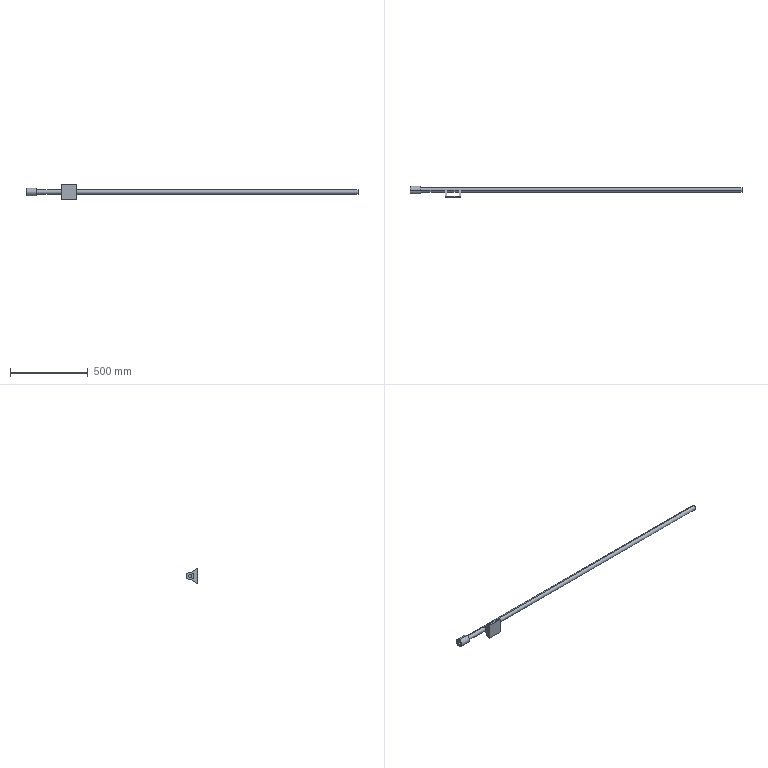Part | STEP file | Rail shaft | 1 solid | 24 faces | box 2134 x 75 x 100 mm | volume 1735049 mm3 | plane 16 | cylinder 8 | commonest cylinder face diameters 30 x4 20 x2 50 x2
STEP:
#1=CARTESIAN_POINT('',(-276.,50.,-10.));
#2=VERTEX_POINT('',#1);
#3=CARTESIAN_POINT('',(-276.,50.,10.));
#4=VERTEX_POINT('',#3);
#5=CARTESIAN_POINT('',(-276.,50.,0.));
#6=DIRECTION('',(-1.,0.,0.));
#7=DIRECTION('',(0.,0.,1.));
#8=AXIS2_PLACEMENT_3D('',#5,#6,#7);
#9=CIRCLE('',#8,10.);
#10=EDGE_CURVE('',#2,#4,#9,.T.);
#11=ORIENTED_EDGE('',*,*,#10,.T.);
#12=CARTESIAN_POINT('',(-256.,50.,10.));
#13=VERTEX_POINT('',#12);
#14=CARTESIAN_POINT('',(-276.,50.,10.));
#15=DIRECTION('',(1.,0.,0.));
#16=VECTOR('',#15,1000.);
#17=LINE('',#14,#16);
#18=EDGE_CURVE('',#4,#13,#17,.T.);
#19=ORIENTED_EDGE('',*,*,#18,.T.);
#20=CARTESIAN_POINT('',(-256.,50.,-10.));
#21=VERTEX_POINT('',#20);
#22=CARTESIAN_POINT('',(-256.,50.,0.));
#23=DIRECTION('',(-1.,0.,0.));
#24=DIRECTION('',(0.,0.,1.));
#25=AXIS2_PLACEMENT_3D('',#22,#23,#24);
#26=CIRCLE('',#25,10.);
#27=EDGE_CURVE('',#21,#13,#26,.T.);
#28=ORIENTED_EDGE('',*,*,#27,.F.);
#29=CARTESIAN_POINT('',(-276.,50.,-10.));
#30=DIRECTION('',(1.,0.,0.));
#31=VECTOR('',#30,1000.);
#32=LINE('',#29,#31);
#33=EDGE_CURVE('',#2,#21,#32,.T.);
#34=ORIENTED_EDGE('',*,*,#33,.F.);
#35=EDGE_LOOP('',(#11,#19,#28,#34));
#36=FACE_OUTER_BOUND('',#35,.T.);
#37=CARTESIAN_POINT('',(-276.,50.,0.));
#38=DIRECTION('',(1.,0.,0.));
#39=DIRECTION('',(0.,0.,-1.));
#40=AXIS2_PLACEMENT_3D('',#37,#38,#39);
#41=CYLINDRICAL_SURFACE('',#40,10.);
#42=ADVANCED_FACE('',(#36),#41,.F.);
#43=CARTESIAN_POINT('',(1858.,50.,-15.));
#44=VERTEX_POINT('',#43);
#45=CARTESIAN_POINT('',(1858.,50.,15.));
#46=VERTEX_POINT('',#45);
#47=CARTESIAN_POINT('',(1858.,50.,0.));
#48=DIRECTION('',(1.,0.,0.));
#49=DIRECTION('',(0.,0.,-1.));
#50=AXIS2_PLACEMENT_3D('',#47,#48,#49);
#51=CIRCLE('',#50,15.);
#52=EDGE_CURVE('',#44,#46,#51,.T.);
#53=ORIENTED_EDGE('',*,*,#52,.F.);
#54=CARTESIAN_POINT('',(50.,50.,-15.));
#55=VERTEX_POINT('',#54);
#56=CARTESIAN_POINT('',(294.,50.,-15.));
#57=DIRECTION('',(-1.,0.,0.));
#58=VECTOR('',#57,1000.);
#59=LINE('',#56,#58);
#60=EDGE_CURVE('',#44,#55,#59,.T.);
#61=ORIENTED_EDGE('',*,*,#60,.T.);
#62=CARTESIAN_POINT('',(40.,50.,-15.));
#63=VERTEX_POINT('',#62);
#64=CARTESIAN_POINT('',(40.,50.,-15.));
#65=DIRECTION('',(1.,0.,0.));
#66=VECTOR('',#65,1000.);
#67=LINE('',#64,#66);
#68=EDGE_CURVE('',#63,#55,#67,.T.);
#69=ORIENTED_EDGE('',*,*,#68,.F.);
#70=CARTESIAN_POINT('',(-40.,50.,-15.));
#71=VERTEX_POINT('',#70);
#72=CARTESIAN_POINT('',(294.,50.,-15.));
#73=DIRECTION('',(-1.,0.,0.));
#74=VECTOR('',#73,1000.);
#75=LINE('',#72,#74);
#76=EDGE_CURVE('',#63,#71,#75,.T.);
#77=ORIENTED_EDGE('',*,*,#76,.T.);
#78=CARTESIAN_POINT('',(-50.,50.,-15.));
#79=VERTEX_POINT('',#78);
#80=CARTESIAN_POINT('',(-40.,50.,-15.));
#81=DIRECTION('',(-1.,0.,0.));
#82=VECTOR('',#81,1000.);
#83=LINE('',#80,#82);
#84=EDGE_CURVE('',#71,#79,#83,.T.);
#85=ORIENTED_EDGE('',*,*,#84,.T.);
#86=CARTESIAN_POINT('',(-206.,50.,-15.));
#87=VERTEX_POINT('',#86);
#88=CARTESIAN_POINT('',(294.,50.,-15.));
#89=DIRECTION('',(-1.,0.,0.));
#90=VECTOR('',#89,1000.);
#91=LINE('',#88,#90);
#92=EDGE_CURVE('',#79,#87,#91,.T.);
#93=ORIENTED_EDGE('',*,*,#92,.T.);
#94=CARTESIAN_POINT('',(-206.,50.,15.));
#95=VERTEX_POINT('',#94);
#96=CARTESIAN_POINT('',(-206.,50.,0.));
#97=DIRECTION('',(-1.,0.,0.));
#98=DIRECTION('',(0.,0.,1.));
#99=AXIS2_PLACEMENT_3D('',#96,#97,#98);
#100=CIRCLE('',#99,15.);
#101=EDGE_CURVE('',#95,#87,#100,.T.);
#102=ORIENTED_EDGE('',*,*,#101,.F.);
#103=CARTESIAN_POINT('',(-50.,50.,15.));
#104=VERTEX_POINT('',#103);
#105=CARTESIAN_POINT('',(294.,50.,15.));
#106=DIRECTION('',(-1.,0.,0.));
#107=VECTOR('',#106,1000.);
#108=LINE('',#105,#107);
#109=EDGE_CURVE('',#104,#95,#108,.T.);
#110=ORIENTED_EDGE('',*,*,#109,.F.);
#111=CARTESIAN_POINT('',(-40.,50.,15.));
#112=VERTEX_POINT('',#111);
#113=CARTESIAN_POINT('',(-40.,50.,15.));
#114=DIRECTION('',(-1.,0.,0.));
#115=VECTOR('',#114,1000.);
#116=LINE('',#113,#115);
#117=EDGE_CURVE('',#112,#104,#116,.T.);
#118=ORIENTED_EDGE('',*,*,#117,.F.);
#119=CARTESIAN_POINT('',(40.,50.,15.));
#120=VERTEX_POINT('',#119);
#121=CARTESIAN_POINT('',(294.,50.,15.));
#122=DIRECTION('',(-1.,0.,0.));
#123=VECTOR('',#122,1000.);
#124=LINE('',#121,#123);
#125=EDGE_CURVE('',#120,#112,#124,.T.);
#126=ORIENTED_EDGE('',*,*,#125,.F.);
#127=CARTESIAN_POINT('',(50.,50.,15.));
#128=VERTEX_POINT('',#127);
#129=CARTESIAN_POINT('',(40.,50.,15.));
#130=DIRECTION('',(1.,0.,0.));
#131=VECTOR('',#130,1000.);
#132=LINE('',#129,#131);
#133=EDGE_CURVE('',#120,#128,#132,.T.);
#134=ORIENTED_EDGE('',*,*,#133,.T.);
#135=CARTESIAN_POINT('',(294.,50.,15.));
#136=DIRECTION('',(-1.,0.,0.));
#137=VECTOR('',#136,1000.);
#138=LINE('',#135,#137);
#139=EDGE_CURVE('',#46,#128,#138,.T.);
#140=ORIENTED_EDGE('',*,*,#139,.F.);
#141=EDGE_LOOP('',(#53,#61,#69,#77,#85,#93,#102,#110,#118,#126,#134,#140));
#142=FACE_OUTER_BOUND('',#141,.T.);
#143=CARTESIAN_POINT('',(294.,50.,0.));
#144=DIRECTION('',(-1.,0.,0.));
#145=DIRECTION('',(0.,0.,1.));
#146=AXIS2_PLACEMENT_3D('',#143,#144,#145);
#147=CYLINDRICAL_SURFACE('',#146,15.);
#148=ADVANCED_FACE('',(#142),#147,.T.);
#149=ORIENTED_EDGE('',*,*,#60,.F.);
#150=CARTESIAN_POINT('',(1858.,50.,0.));
#151=DIRECTION('',(1.,0.,0.));
#152=DIRECTION('',(0.,0.,-1.));
#153=AXIS2_PLACEMENT_3D('',#150,#151,#152);
#154=CIRCLE('',#153,15.);
#155=EDGE_CURVE('',#46,#44,#154,.T.);
#156=ORIENTED_EDGE('',*,*,#155,.F.);
#157=ORIENTED_EDGE('',*,*,#139,.T.);
#158=CARTESIAN_POINT('',(50.,50.,0.));
#159=DIRECTION('',(1.,0.,0.));
#160=DIRECTION('',(0.,0.,-1.));
#161=AXIS2_PLACEMENT_3D('',#158,#159,#160);
#162=CIRCLE('',#161,15.);
#163=EDGE_CURVE('',#128,#55,#162,.T.);
#164=ORIENTED_EDGE('',*,*,#163,.T.);
#165=EDGE_LOOP('',(#149,#156,#157,#164));
#166=FACE_OUTER_BOUND('',#165,.T.);
#167=CARTESIAN_POINT('',(294.,50.,0.));
#168=DIRECTION('',(-1.,0.,0.));
#169=DIRECTION('',(0.,0.,1.));
#170=AXIS2_PLACEMENT_3D('',#167,#168,#169);
#171=CYLINDRICAL_SURFACE('',#170,15.);
#172=ADVANCED_FACE('',(#166),#171,.T.);
#173=ORIENTED_EDGE('',*,*,#76,.F.);
#174=CARTESIAN_POINT('',(40.,50.,0.));
#175=DIRECTION('',(-1.,0.,0.));
#176=DIRECTION('',(0.,0.,1.));
#177=AXIS2_PLACEMENT_3D('',#174,#175,#176);
#178=CIRCLE('',#177,15.);
#179=EDGE_CURVE('',#63,#120,#178,.T.);
#180=ORIENTED_EDGE('',*,*,#179,.T.);
#181=ORIENTED_EDGE('',*,*,#125,.T.);
#182=CARTESIAN_POINT('',(-40.,50.,0.));
#183=DIRECTION('',(-1.,0.,0.));
#184=DIRECTION('',(0.,0.,-1.));
#185=AXIS2_PLACEMENT_3D('',#182,#183,#184);
#186=CIRCLE('',#185,15.);
#187=EDGE_CURVE('',#71,#112,#186,.T.);
#188=ORIENTED_EDGE('',*,*,#187,.F.);
#189=EDGE_LOOP('',(#173,#180,#181,#188));
#190=FACE_OUTER_BOUND('',#189,.T.);
#191=CARTESIAN_POINT('',(294.,50.,0.));
#192=DIRECTION('',(-1.,0.,0.));
#193=DIRECTION('',(0.,0.,1.));
#194=AXIS2_PLACEMENT_3D('',#191,#192,#193);
#195=CYLINDRICAL_SURFACE('',#194,15.);
#196=ADVANCED_FACE('',(#190),#195,.T.);
#197=CARTESIAN_POINT('',(-276.,50.,25.));
#198=VERTEX_POINT('',#197);
#199=CARTESIAN_POINT('',(-276.,50.,-25.));
#200=VERTEX_POINT('',#199);
#201=CARTESIAN_POINT('',(-276.,50.,0.));
#202=DIRECTION('',(-1.,0.,0.));
#203=DIRECTION('',(0.,0.,1.));
#204=AXIS2_PLACEMENT_3D('',#201,#202,#203);
#205=CIRCLE('',#204,25.);
#206=EDGE_CURVE('',#198,#200,#205,.T.);
#207=ORIENTED_EDGE('',*,*,#206,.F.);
#208=CARTESIAN_POINT('',(-206.,50.,25.));
#209=VERTEX_POINT('',#208);
#210=CARTESIAN_POINT('',(-256.,50.,25.));
#211=DIRECTION('',(1.,0.,0.));
#212=VECTOR('',#211,1000.);
#213=LINE('',#210,#212);
#214=EDGE_CURVE('',#198,#209,#213,.T.);
#215=ORIENTED_EDGE('',*,*,#214,.T.);
#216=CARTESIAN_POINT('',(-206.,50.,-25.));
#217=VERTEX_POINT('',#216);
#218=CARTESIAN_POINT('',(-206.,50.,0.));
#219=DIRECTION('',(-1.,0.,0.));
#220=DIRECTION('',(0.,0.,1.));
#221=AXIS2_PLACEMENT_3D('',#218,#219,#220);
#222=CIRCLE('',#221,25.);
#223=EDGE_CURVE('',#209,#217,#222,.T.);
#224=ORIENTED_EDGE('',*,*,#223,.T.);
#225=CARTESIAN_POINT('',(-256.,50.,-25.));
#226=DIRECTION('',(1.,0.,0.));
#227=VECTOR('',#226,1000.);
#228=LINE('',#225,#227);
#229=EDGE_CURVE('',#200,#217,#228,.T.);
#230=ORIENTED_EDGE('',*,*,#229,.F.);
#231=EDGE_LOOP('',(#207,#215,#224,#230));
#232=FACE_OUTER_BOUND('',#231,.T.);
#233=CARTESIAN_POINT('',(-256.,50.,0.));
#234=DIRECTION('',(1.,0.,0.));
#235=DIRECTION('',(0.,0.,-1.));
#236=AXIS2_PLACEMENT_3D('',#233,#234,#235);
#237=CYLINDRICAL_SURFACE('',#236,25.);
#238=ADVANCED_FACE('',(#232),#237,.T.);
#239=CARTESIAN_POINT('',(-40.,10.,50.));
#240=VERTEX_POINT('',#239);
#241=CARTESIAN_POINT('',(-40.,10.,-50.));
#242=VERTEX_POINT('',#241);
#243=CARTESIAN_POINT('',(-40.,10.,50.));
#244=DIRECTION('',(0.,0.,-1.));
#245=VECTOR('',#244,1000.);
#246=LINE('',#243,#245);
#247=EDGE_CURVE('',#240,#242,#246,.T.);
#248=ORIENTED_EDGE('',*,*,#247,.F.);
#249=CARTESIAN_POINT('',(40.,10.,50.));
#250=VERTEX_POINT('',#249);
#251=CARTESIAN_POINT('',(-50.,10.,50.));
#252=DIRECTION('',(1.,0.,0.));
#253=VECTOR('',#252,1000.);
#254=LINE('',#251,#253);
#255=EDGE_CURVE('',#240,#250,#254,.T.);
#256=ORIENTED_EDGE('',*,*,#255,.T.);
#257=CARTESIAN_POINT('',(40.,10.,-50.));
#258=VERTEX_POINT('',#257);
#259=CARTESIAN_POINT('',(40.,10.,50.));
#260=DIRECTION('',(0.,0.,-1.));
#261=VECTOR('',#260,1000.);
#262=LINE('',#259,#261);
#263=EDGE_CURVE('',#250,#258,#262,.T.);
#264=ORIENTED_EDGE('',*,*,#263,.T.);
#265=CARTESIAN_POINT('',(-50.,10.,-50.));
#266=DIRECTION('',(-1.,0.,0.));
#267=VECTOR('',#266,1000.);
#268=LINE('',#265,#267);
#269=EDGE_CURVE('',#258,#242,#268,.T.);
#270=ORIENTED_EDGE('',*,*,#269,.T.);
#271=EDGE_LOOP('',(#248,#256,#264,#270));
#272=FACE_OUTER_BOUND('',#271,.T.);
#273=CARTESIAN_POINT('',(0.,10.,0.));
#274=DIRECTION('',(0.,1.,0.));
#275=DIRECTION('',(0.,0.,1.));
#276=AXIS2_PLACEMENT_3D('',#273,#274,#275);
#277=PLANE('',#276);
#278=ADVANCED_FACE('',(#272),#277,.T.);
#279=ORIENTED_EDGE('',*,*,#163,.F.);
#280=CARTESIAN_POINT('',(50.,10.,50.));
#281=VERTEX_POINT('',#280);
#282=CARTESIAN_POINT('',(50.,50.,15.));
#283=DIRECTION('',(0.,-0.7526,0.6585));
#284=VECTOR('',#283,1000.);
#285=LINE('',#282,#284);
#286=EDGE_CURVE('',#128,#281,#285,.T.);
#287=ORIENTED_EDGE('',*,*,#286,.T.);
#288=CARTESIAN_POINT('',(50.,0.,50.));
#289=VERTEX_POINT('',#288);
#290=CARTESIAN_POINT('',(50.,10.,50.));
#291=DIRECTION('',(0.,-1.,0.));
#292=VECTOR('',#291,1000.);
#293=LINE('',#290,#292);
#294=EDGE_CURVE('',#281,#289,#293,.T.);
#295=ORIENTED_EDGE('',*,*,#294,.T.);
#296=CARTESIAN_POINT('',(50.,0.,-50.));
#297=VERTEX_POINT('',#296);
#298=CARTESIAN_POINT('',(50.,0.,-50.));
#299=DIRECTION('',(0.,0.,-1.));
#300=VECTOR('',#299,1000.);
#301=LINE('',#298,#300);
#302=EDGE_CURVE('',#289,#297,#301,.T.);
#303=ORIENTED_EDGE('',*,*,#302,.T.);
#304=CARTESIAN_POINT('',(50.,10.,-50.));
#305=VERTEX_POINT('',#304);
#306=CARTESIAN_POINT('',(50.,10.,-50.));
#307=DIRECTION('',(0.,-1.,0.));
#308=VECTOR('',#307,1000.);
#309=LINE('',#306,#308);
#310=EDGE_CURVE('',#305,#297,#309,.T.);
#311=ORIENTED_EDGE('',*,*,#310,.F.);
#312=CARTESIAN_POINT('',(50.,10.,-50.));
#313=DIRECTION('',(0.,0.7526,0.6585));
#314=VECTOR('',#313,1000.);
#315=LINE('',#312,#314);
#316=EDGE_CURVE('',#305,#55,#315,.T.);
#317=ORIENTED_EDGE('',*,*,#316,.T.);
#318=EDGE_LOOP('',(#279,#287,#295,#303,#311,#317));
#319=FACE_OUTER_BOUND('',#318,.T.);
#320=CARTESIAN_POINT('',(50.,10.,-50.));
#321=DIRECTION('',(-1.,0.,0.));
#322=DIRECTION('',(0.,0.,1.));
#323=AXIS2_PLACEMENT_3D('',#320,#321,#322);
#324=PLANE('',#323);
#325=ADVANCED_FACE('',(#319),#324,.F.);
#326=CARTESIAN_POINT('',(-50.,0.,-50.));
#327=VERTEX_POINT('',#326);
#328=CARTESIAN_POINT('',(-50.,0.,-50.));
#329=DIRECTION('',(-1.,0.,0.));
#330=VECTOR('',#329,1000.);
#331=LINE('',#328,#330);
#332=EDGE_CURVE('',#297,#327,#331,.T.);
#333=ORIENTED_EDGE('',*,*,#332,.T.);
#334=CARTESIAN_POINT('',(-50.,10.,-50.));
#335=VERTEX_POINT('',#334);
#336=CARTESIAN_POINT('',(-50.,10.,-50.));
#337=DIRECTION('',(0.,-1.,0.));
#338=VECTOR('',#337,1000.);
#339=LINE('',#336,#338);
#340=EDGE_CURVE('',#335,#327,#339,.T.);
#341=ORIENTED_EDGE('',*,*,#340,.F.);
#342=CARTESIAN_POINT('',(-40.,10.,-50.));
#343=DIRECTION('',(-1.,0.,0.));
#344=VECTOR('',#343,1000.);
#345=LINE('',#342,#344);
#346=EDGE_CURVE('',#242,#335,#345,.T.);
#347=ORIENTED_EDGE('',*,*,#346,.F.);
#348=ORIENTED_EDGE('',*,*,#269,.F.);
#349=CARTESIAN_POINT('',(-50.,10.,-50.));
#350=DIRECTION('',(-1.,0.,0.));
#351=VECTOR('',#350,1000.);
#352=LINE('',#349,#351);
#353=EDGE_CURVE('',#305,#258,#352,.T.);
#354=ORIENTED_EDGE('',*,*,#353,.F.);
#355=ORIENTED_EDGE('',*,*,#310,.T.);
#356=EDGE_LOOP('',(#333,#341,#347,#348,#354,#355));
#357=FACE_OUTER_BOUND('',#356,.T.);
#358=CARTESIAN_POINT('',(-50.,10.,-50.));
#359=DIRECTION('',(0.,0.,1.));
#360=DIRECTION('',(1.,0.,0.));
#361=AXIS2_PLACEMENT_3D('',#358,#359,#360);
#362=PLANE('',#361);
#363=ADVANCED_FACE('',(#357),#362,.F.);
#364=CARTESIAN_POINT('',(-50.,0.,50.));
#365=VERTEX_POINT('',#364);
#366=CARTESIAN_POINT('',(-50.,0.,-50.));
#367=DIRECTION('',(0.,0.,1.));
#368=VECTOR('',#367,1000.);
#369=LINE('',#366,#368);
#370=EDGE_CURVE('',#327,#365,#369,.T.);
#371=ORIENTED_EDGE('',*,*,#370,.T.);
#372=CARTESIAN_POINT('',(-50.,10.,50.));
#373=VERTEX_POINT('',#372);
#374=CARTESIAN_POINT('',(-50.,10.,50.));
#375=DIRECTION('',(0.,-1.,0.));
#376=VECTOR('',#375,1000.);
#377=LINE('',#374,#376);
#378=EDGE_CURVE('',#373,#365,#377,.T.);
#379=ORIENTED_EDGE('',*,*,#378,.F.);
#380=CARTESIAN_POINT('',(-50.,50.,15.));
#381=DIRECTION('',(0.,-0.7526,0.6585));
#382=VECTOR('',#381,1000.);
#383=LINE('',#380,#382);
#384=EDGE_CURVE('',#104,#373,#383,.T.);
#385=ORIENTED_EDGE('',*,*,#384,.F.);
#386=CARTESIAN_POINT('',(-50.,50.,0.));
#387=DIRECTION('',(-1.,0.,0.));
#388=DIRECTION('',(0.,0.,-1.));
#389=AXIS2_PLACEMENT_3D('',#386,#387,#388);
#390=CIRCLE('',#389,15.);
#391=EDGE_CURVE('',#79,#104,#390,.T.);
#392=ORIENTED_EDGE('',*,*,#391,.F.);
#393=CARTESIAN_POINT('',(-50.,10.,-50.));
#394=DIRECTION('',(0.,0.7526,0.6585));
#395=VECTOR('',#394,1000.);
#396=LINE('',#393,#395);
#397=EDGE_CURVE('',#335,#79,#396,.T.);
#398=ORIENTED_EDGE('',*,*,#397,.F.);
#399=ORIENTED_EDGE('',*,*,#340,.T.);
#400=EDGE_LOOP('',(#371,#379,#385,#392,#398,#399));
#401=FACE_OUTER_BOUND('',#400,.T.);
#402=CARTESIAN_POINT('',(-50.,10.,-50.));
#403=DIRECTION('',(1.,0.,0.));
#404=DIRECTION('',(0.,0.,-1.));
#405=AXIS2_PLACEMENT_3D('',#402,#403,#404);
#406=PLANE('',#405);
#407=ADVANCED_FACE('',(#401),#406,.F.);
#408=CARTESIAN_POINT('',(-50.,0.,50.));
#409=DIRECTION('',(1.,0.,0.));
#410=VECTOR('',#409,1000.);
#411=LINE('',#408,#410);
#412=EDGE_CURVE('',#365,#289,#411,.T.);
#413=ORIENTED_EDGE('',*,*,#412,.T.);
#414=ORIENTED_EDGE('',*,*,#294,.F.);
#415=CARTESIAN_POINT('',(40.,10.,50.));
#416=DIRECTION('',(1.,0.,0.));
#417=VECTOR('',#416,1000.);
#418=LINE('',#415,#417);
#419=EDGE_CURVE('',#250,#281,#418,.T.);
#420=ORIENTED_EDGE('',*,*,#419,.F.);
#421=ORIENTED_EDGE('',*,*,#255,.F.);
#422=CARTESIAN_POINT('',(-50.,10.,50.));
#423=DIRECTION('',(1.,0.,0.));
#424=VECTOR('',#423,1000.);
#425=LINE('',#422,#424);
#426=EDGE_CURVE('',#373,#240,#425,.T.);
#427=ORIENTED_EDGE('',*,*,#426,.F.);
#428=ORIENTED_EDGE('',*,*,#378,.T.);
#429=EDGE_LOOP('',(#413,#414,#420,#421,#427,#428));
#430=FACE_OUTER_BOUND('',#429,.T.);
#431=CARTESIAN_POINT('',(-50.,10.,50.));
#432=DIRECTION('',(0.,0.,-1.));
#433=DIRECTION('',(-1.,0.,0.));
#434=AXIS2_PLACEMENT_3D('',#431,#432,#433);
#435=PLANE('',#434);
#436=ADVANCED_FACE('',(#430),#435,.F.);
#437=ORIENTED_EDGE('',*,*,#302,.F.);
#438=ORIENTED_EDGE('',*,*,#412,.F.);
#439=ORIENTED_EDGE('',*,*,#370,.F.);
#440=ORIENTED_EDGE('',*,*,#332,.F.);
#441=EDGE_LOOP('',(#437,#438,#439,#440));
#442=FACE_OUTER_BOUND('',#441,.T.);
#443=CARTESIAN_POINT('',(0.,0.,0.));
#444=DIRECTION('',(0.,1.,0.));
#445=DIRECTION('',(0.,0.,1.));
#446=AXIS2_PLACEMENT_3D('',#443,#444,#445);
#447=PLANE('',#446);
#448=ADVANCED_FACE('',(#442),#447,.F.);
#449=ORIENTED_EDGE('',*,*,#286,.F.);
#450=ORIENTED_EDGE('',*,*,#133,.F.);
#451=CARTESIAN_POINT('',(40.,50.,15.));
#452=DIRECTION('',(0.,-0.7526,0.6585));
#453=VECTOR('',#452,1000.);
#454=LINE('',#451,#453);
#455=EDGE_CURVE('',#120,#250,#454,.T.);
#456=ORIENTED_EDGE('',*,*,#455,.T.);
#457=ORIENTED_EDGE('',*,*,#419,.T.);
#458=EDGE_LOOP('',(#449,#450,#456,#457));
#459=FACE_OUTER_BOUND('',#458,.T.);
#460=CARTESIAN_POINT('',(40.,50.,15.));
#461=DIRECTION('',(0.,0.6585,0.7526));
#462=DIRECTION('',(0.,-0.7526,0.6585));
#463=AXIS2_PLACEMENT_3D('',#460,#461,#462);
#464=PLANE('',#463);
#465=ADVANCED_FACE('',(#459),#464,.T.);
#466=ORIENTED_EDGE('',*,*,#316,.F.);
#467=ORIENTED_EDGE('',*,*,#353,.T.);
#468=CARTESIAN_POINT('',(40.,10.,-50.));
#469=DIRECTION('',(0.,0.7526,0.6585));
#470=VECTOR('',#469,1000.);
#471=LINE('',#468,#470);
#472=EDGE_CURVE('',#258,#63,#471,.T.);
#473=ORIENTED_EDGE('',*,*,#472,.T.);
#474=ORIENTED_EDGE('',*,*,#68,.T.);
#475=EDGE_LOOP('',(#466,#467,#473,#474));
#476=FACE_OUTER_BOUND('',#475,.T.);
#477=CARTESIAN_POINT('',(40.,10.,-50.));
#478=DIRECTION('',(0.,0.6585,-0.7526));
#479=DIRECTION('',(0.,0.7526,0.6585));
#480=AXIS2_PLACEMENT_3D('',#477,#478,#479);
#481=PLANE('',#480);
#482=ADVANCED_FACE('',(#476),#481,.T.);
#483=ORIENTED_EDGE('',*,*,#179,.F.);
#484=ORIENTED_EDGE('',*,*,#472,.F.);
#485=ORIENTED_EDGE('',*,*,#263,.F.);
#486=ORIENTED_EDGE('',*,*,#455,.F.);
#487=EDGE_LOOP('',(#483,#484,#485,#486));
#488=FACE_OUTER_BOUND('',#487,.T.);
#489=CARTESIAN_POINT('',(40.,0.,0.));
#490=DIRECTION('',(-1.,0.,0.));
#491=DIRECTION('',(0.,0.,1.));
#492=AXIS2_PLACEMENT_3D('',#489,#490,#491);
#493=PLANE('',#492);
#494=ADVANCED_FACE('',(#488),#493,.T.);
#495=ORIENTED_EDGE('',*,*,#214,.F.);
#496=CARTESIAN_POINT('',(-276.,50.,0.));
#497=DIRECTION('',(-1.,0.,0.));
#498=DIRECTION('',(0.,0.,1.));
#499=AXIS2_PLACEMENT_3D('',#496,#497,#498);
#500=CIRCLE('',#499,25.);
#501=EDGE_CURVE('',#200,#198,#500,.T.);
#502=ORIENTED_EDGE('',*,*,#501,.F.);
#503=ORIENTED_EDGE('',*,*,#229,.T.);
#504=CARTESIAN_POINT('',(-206.,50.,0.));
#505=DIRECTION('',(-1.,0.,0.));
#506=DIRECTION('',(0.,0.,1.));
#507=AXIS2_PLACEMENT_3D('',#504,#505,#506);
#508=CIRCLE('',#507,25.);
#509=EDGE_CURVE('',#217,#209,#508,.T.);
#510=ORIENTED_EDGE('',*,*,#509,.T.);
#511=EDGE_LOOP('',(#495,#502,#503,#510));
#512=FACE_OUTER_BOUND('',#511,.T.);
#513=CARTESIAN_POINT('',(-256.,50.,0.));
#514=DIRECTION('',(1.,0.,0.));
#515=DIRECTION('',(0.,0.,-1.));
#516=AXIS2_PLACEMENT_3D('',#513,#514,#515);
#517=CYLINDRICAL_SURFACE('',#516,25.);
#518=ADVANCED_FACE('',(#512),#517,.T.);
#519=ORIENTED_EDGE('',*,*,#101,.T.);
#520=CARTESIAN_POINT('',(-206.,50.,0.));
#521=DIRECTION('',(-1.,0.,0.));
#522=DIRECTION('',(0.,0.,1.));
#523=AXIS2_PLACEMENT_3D('',#520,#521,#522);
#524=CIRCLE('',#523,15.);
#525=EDGE_CURVE('',#87,#95,#524,.T.);
#526=ORIENTED_EDGE('',*,*,#525,.T.);
#527=EDGE_LOOP('',(#519,#526));
#528=FACE_BOUND('',#527,.T.);
#529=ORIENTED_EDGE('',*,*,#509,.F.);
#530=ORIENTED_EDGE('',*,*,#223,.F.);
#531=EDGE_LOOP('',(#529,#530));
#532=FACE_OUTER_BOUND('',#531,.T.);
#533=CARTESIAN_POINT('',(-206.,50.,0.));
#534=DIRECTION('',(-1.,0.,0.));
#535=DIRECTION('',(0.,0.,1.));
#536=AXIS2_PLACEMENT_3D('',#533,#534,#535);
#537=PLANE('',#536);
#538=ADVANCED_FACE('',(#528,#532),#537,.F.);
#539=ORIENTED_EDGE('',*,*,#92,.F.);
#540=ORIENTED_EDGE('',*,*,#391,.T.);
#541=ORIENTED_EDGE('',*,*,#109,.T.);
#542=ORIENTED_EDGE('',*,*,#525,.F.);
#543=EDGE_LOOP('',(#539,#540,#541,#542));
#544=FACE_OUTER_BOUND('',#543,.T.);
#545=CARTESIAN_POINT('',(294.,50.,0.));
#546=DIRECTION('',(-1.,0.,0.));
#547=DIRECTION('',(0.,0.,1.));
#548=AXIS2_PLACEMENT_3D('',#545,#546,#547);
#549=CYLINDRICAL_SURFACE('',#548,15.);
#550=ADVANCED_FACE('',(#544),#549,.T.);
#551=ORIENTED_EDGE('',*,*,#384,.T.);
#552=ORIENTED_EDGE('',*,*,#426,.T.);
#553=CARTESIAN_POINT('',(-40.,50.,15.));
#554=DIRECTION('',(0.,-0.7526,0.6585));
#555=VECTOR('',#554,1000.);
#556=LINE('',#553,#555);
#557=EDGE_CURVE('',#112,#240,#556,.T.);
#558=ORIENTED_EDGE('',*,*,#557,.F.);
#559=ORIENTED_EDGE('',*,*,#117,.T.);
#560=EDGE_LOOP('',(#551,#552,#558,#559));
#561=FACE_OUTER_BOUND('',#560,.T.);
#562=CARTESIAN_POINT('',(-40.,50.,15.));
#563=DIRECTION('',(0.,-0.6585,-0.7526));
#564=DIRECTION('',(0.,0.7526,-0.6585));
#565=AXIS2_PLACEMENT_3D('',#562,#563,#564);
#566=PLANE('',#565);
#567=ADVANCED_FACE('',(#561),#566,.F.);
#568=ORIENTED_EDGE('',*,*,#397,.T.);
#569=ORIENTED_EDGE('',*,*,#84,.F.);
#570=CARTESIAN_POINT('',(-40.,10.,-50.));
#571=DIRECTION('',(0.,0.7526,0.6585));
#572=VECTOR('',#571,1000.);
#573=LINE('',#570,#572);
#574=EDGE_CURVE('',#242,#71,#573,.T.);
#575=ORIENTED_EDGE('',*,*,#574,.F.);
#576=ORIENTED_EDGE('',*,*,#346,.T.);
#577=EDGE_LOOP('',(#568,#569,#575,#576));
#578=FACE_OUTER_BOUND('',#577,.T.);
#579=CARTESIAN_POINT('',(-40.,10.,-50.));
#580=DIRECTION('',(0.,-0.6585,0.7526));
#581=DIRECTION('',(0.,-0.7526,-0.6585));
#582=AXIS2_PLACEMENT_3D('',#579,#580,#581);
#583=PLANE('',#582);
#584=ADVANCED_FACE('',(#578),#583,.F.);
#585=ORIENTED_EDGE('',*,*,#574,.T.);
#586=ORIENTED_EDGE('',*,*,#187,.T.);
#587=ORIENTED_EDGE('',*,*,#557,.T.);
#588=ORIENTED_EDGE('',*,*,#247,.T.);
#589=EDGE_LOOP('',(#585,#586,#587,#588));
#590=FACE_OUTER_BOUND('',#589,.T.);
#591=CARTESIAN_POINT('',(-40.,0.,0.));
#592=DIRECTION('',(1.,0.,0.));
#593=DIRECTION('',(0.,0.,1.));
#594=AXIS2_PLACEMENT_3D('',#591,#592,#593);
#595=PLANE('',#594);
#596=ADVANCED_FACE('',(#590),#595,.T.);
#597=ORIENTED_EDGE('',*,*,#501,.T.);
#598=ORIENTED_EDGE('',*,*,#206,.T.);
#599=EDGE_LOOP('',(#597,#598));
#600=FACE_OUTER_BOUND('',#599,.T.);
#601=ORIENTED_EDGE('',*,*,#10,.F.);
#602=CARTESIAN_POINT('',(-276.,50.,0.));
#603=DIRECTION('',(-1.,0.,0.));
#604=DIRECTION('',(0.,0.,1.));
#605=AXIS2_PLACEMENT_3D('',#602,#603,#604);
#606=CIRCLE('',#605,10.);
#607=EDGE_CURVE('',#4,#2,#606,.T.);
#608=ORIENTED_EDGE('',*,*,#607,.F.);
#609=EDGE_LOOP('',(#601,#608));
#610=FACE_BOUND('',#609,.T.);
#611=CARTESIAN_POINT('',(-276.,50.,0.));
#612=DIRECTION('',(-1.,0.,0.));
#613=DIRECTION('',(0.,0.,1.));
#614=AXIS2_PLACEMENT_3D('',#611,#612,#613);
#615=PLANE('',#614);
#616=ADVANCED_FACE('',(#600,#610),#615,.T.);
#617=ORIENTED_EDGE('',*,*,#18,.F.);
#618=ORIENTED_EDGE('',*,*,#607,.T.);
#619=ORIENTED_EDGE('',*,*,#33,.T.);
#620=CARTESIAN_POINT('',(-256.,50.,0.));
#621=DIRECTION('',(-1.,0.,0.));
#622=DIRECTION('',(0.,0.,1.));
#623=AXIS2_PLACEMENT_3D('',#620,#621,#622);
#624=CIRCLE('',#623,10.);
#625=EDGE_CURVE('',#13,#21,#624,.T.);
#626=ORIENTED_EDGE('',*,*,#625,.F.);
#627=EDGE_LOOP('',(#617,#618,#619,#626));
#628=FACE_OUTER_BOUND('',#627,.T.);
#629=CARTESIAN_POINT('',(-276.,50.,0.));
#630=DIRECTION('',(1.,0.,0.));
#631=DIRECTION('',(0.,0.,-1.));
#632=AXIS2_PLACEMENT_3D('',#629,#630,#631);
#633=CYLINDRICAL_SURFACE('',#632,10.);
#634=ADVANCED_FACE('',(#628),#633,.F.);
#635=ORIENTED_EDGE('',*,*,#27,.T.);
#636=ORIENTED_EDGE('',*,*,#625,.T.);
#637=EDGE_LOOP('',(#635,#636));
#638=FACE_OUTER_BOUND('',#637,.T.);
#639=CARTESIAN_POINT('',(-256.,50.,0.));
#640=DIRECTION('',(1.,0.,0.));
#641=DIRECTION('',(0.,0.,-1.));
#642=AXIS2_PLACEMENT_3D('',#639,#640,#641);
#643=PLANE('',#642);
#644=ADVANCED_FACE('',(#638),#643,.F.);
#645=ORIENTED_EDGE('',*,*,#155,.T.);
#646=ORIENTED_EDGE('',*,*,#52,.T.);
#647=EDGE_LOOP('',(#645,#646));
#648=FACE_OUTER_BOUND('',#647,.T.);
#649=CARTESIAN_POINT('',(1858.,10.,-50.));
#650=DIRECTION('',(1.,0.,0.));
#651=DIRECTION('',(0.,0.,1.));
#652=AXIS2_PLACEMENT_3D('',#649,#650,#651);
#653=PLANE('',#652);
#654=ADVANCED_FACE('',(#648),#653,.T.);
#655=CLOSED_SHELL('',(#42,#148,#172,#196,#238,#278,#325,#363,#407,#436,#448,#465,#482,#494,#518,#538,#550,#567,#584,#596,#616,#634,#644,#654));
#656=MANIFOLD_SOLID_BREP('',#655);
#657=CARTESIAN_POINT('',(0.,0.,0.));
#658=DIRECTION('',(0.,0.,1.));
#659=DIRECTION('',(1.,0.,0.));
#660=AXIS2_PLACEMENT_3D('',#657,#658,#659);
#661=(LENGTH_UNIT()NAMED_UNIT(*)SI_UNIT(.MILLI.,.METRE.));
#662=UNCERTAINTY_MEASURE_WITH_UNIT(LENGTH_MEASURE(0.00001),#661,'','');
#663=(NAMED_UNIT(*)PLANE_ANGLE_UNIT()SI_UNIT($,.RADIAN.));
#664=(NAMED_UNIT(*)SI_UNIT($,.STERADIAN.)SOLID_ANGLE_UNIT());
#665=(GEOMETRIC_REPRESENTATION_CONTEXT(3)GLOBAL_UNCERTAINTY_ASSIGNED_CONTEXT((#662))GLOBAL_UNIT_ASSIGNED_CONTEXT((#661,#663,#664))REPRESENTATION_CONTEXT('',''));
#666=ADVANCED_BREP_SHAPE_REPRESENTATION('',(#656,#660),#665);